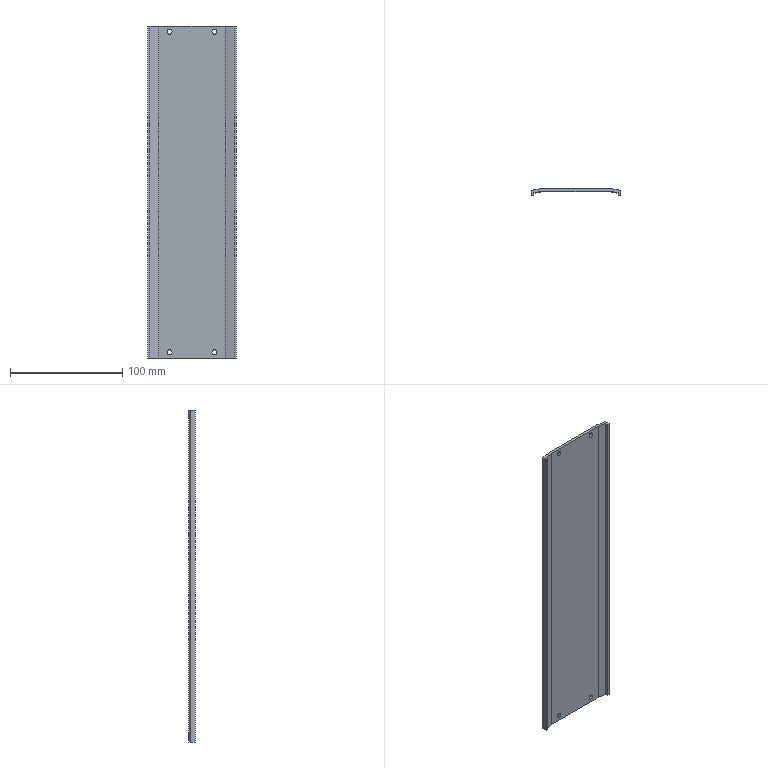Part | SolidWorks | features Cut 1, Extrusion 1, MirrorPattern 1 | 1 solid | 22 faces | box 79 x 6 x 296 mm | volume 60805 mm3 | plane 14 | cylinder 8 | commonest cylinder face diameters 4.5 x8
STEP:
#1=CARTESIAN_POINT('',(20.,3.5,-140.75));
#2=VERTEX_POINT('',#1);
#3=CARTESIAN_POINT('',(20.,3.5,-145.25));
#4=VERTEX_POINT('',#3);
#5=CARTESIAN_POINT('',(20.,3.5,-143.));
#6=DIRECTION('',(0.,-1.,0.));
#7=DIRECTION('',(0.,0.,1.));
#8=AXIS2_PLACEMENT_3D('',#5,#6,#7);
#9=CIRCLE('',#8,2.25);
#10=EDGE_CURVE('',#2,#4,#9,.T.);
#11=ORIENTED_EDGE('',*,*,#10,.T.);
#12=CARTESIAN_POINT('',(20.,6.,-145.25));
#13=VERTEX_POINT('',#12);
#14=CARTESIAN_POINT('',(20.,-4.,-145.25));
#15=DIRECTION('',(0.,1.,0.));
#16=VECTOR('',#15,1000.);
#17=LINE('',#14,#16);
#18=EDGE_CURVE('',#4,#13,#17,.T.);
#19=ORIENTED_EDGE('',*,*,#18,.T.);
#20=CARTESIAN_POINT('',(20.,6.,-140.75));
#21=VERTEX_POINT('',#20);
#22=CARTESIAN_POINT('',(20.,6.,-143.));
#23=DIRECTION('',(0.,-1.,0.));
#24=DIRECTION('',(0.,0.,-1.));
#25=AXIS2_PLACEMENT_3D('',#22,#23,#24);
#26=CIRCLE('',#25,2.25);
#27=EDGE_CURVE('',#21,#13,#26,.T.);
#28=ORIENTED_EDGE('',*,*,#27,.F.);
#29=CARTESIAN_POINT('',(20.,-4.,-140.75));
#30=DIRECTION('',(0.,1.,0.));
#31=VECTOR('',#30,1000.);
#32=LINE('',#29,#31);
#33=EDGE_CURVE('',#2,#21,#32,.T.);
#34=ORIENTED_EDGE('',*,*,#33,.F.);
#35=EDGE_LOOP('',(#11,#19,#28,#34));
#36=FACE_OUTER_BOUND('',#35,.T.);
#37=CARTESIAN_POINT('',(20.,-4.,-143.));
#38=DIRECTION('',(0.,1.,0.));
#39=DIRECTION('',(0.,0.,1.));
#40=AXIS2_PLACEMENT_3D('',#37,#38,#39);
#41=CYLINDRICAL_SURFACE('',#40,2.25);
#42=ADVANCED_FACE('',(#36),#41,.F.);
#43=CARTESIAN_POINT('',(-20.,3.5,-140.75));
#44=VERTEX_POINT('',#43);
#45=CARTESIAN_POINT('',(-20.,3.5,-145.25));
#46=VERTEX_POINT('',#45);
#47=CARTESIAN_POINT('',(-20.,3.5,-143.));
#48=DIRECTION('',(0.,-1.,0.));
#49=DIRECTION('',(0.,0.,1.));
#50=AXIS2_PLACEMENT_3D('',#47,#48,#49);
#51=CIRCLE('',#50,2.25);
#52=EDGE_CURVE('',#44,#46,#51,.T.);
#53=ORIENTED_EDGE('',*,*,#52,.T.);
#54=CARTESIAN_POINT('',(-20.,6.,-145.25));
#55=VERTEX_POINT('',#54);
#56=CARTESIAN_POINT('',(-20.,-4.,-145.25));
#57=DIRECTION('',(0.,1.,0.));
#58=VECTOR('',#57,1000.);
#59=LINE('',#56,#58);
#60=EDGE_CURVE('',#46,#55,#59,.T.);
#61=ORIENTED_EDGE('',*,*,#60,.T.);
#62=CARTESIAN_POINT('',(-20.,6.,-140.75));
#63=VERTEX_POINT('',#62);
#64=CARTESIAN_POINT('',(-20.,6.,-143.));
#65=DIRECTION('',(0.,-1.,0.));
#66=DIRECTION('',(0.,0.,-1.));
#67=AXIS2_PLACEMENT_3D('',#64,#65,#66);
#68=CIRCLE('',#67,2.25);
#69=EDGE_CURVE('',#63,#55,#68,.T.);
#70=ORIENTED_EDGE('',*,*,#69,.F.);
#71=CARTESIAN_POINT('',(-20.,-4.,-140.75));
#72=DIRECTION('',(0.,1.,0.));
#73=VECTOR('',#72,1000.);
#74=LINE('',#71,#73);
#75=EDGE_CURVE('',#44,#63,#74,.T.);
#76=ORIENTED_EDGE('',*,*,#75,.F.);
#77=EDGE_LOOP('',(#53,#61,#70,#76));
#78=FACE_OUTER_BOUND('',#77,.T.);
#79=CARTESIAN_POINT('',(-20.,-4.,-143.));
#80=DIRECTION('',(0.,1.,0.));
#81=DIRECTION('',(0.,0.,1.));
#82=AXIS2_PLACEMENT_3D('',#79,#80,#81);
#83=CYLINDRICAL_SURFACE('',#82,2.25);
#84=ADVANCED_FACE('',(#78),#83,.F.);
#85=CARTESIAN_POINT('',(20.,3.5,140.75));
#86=VERTEX_POINT('',#85);
#87=CARTESIAN_POINT('',(20.,3.5,145.25));
#88=VERTEX_POINT('',#87);
#89=CARTESIAN_POINT('',(20.,3.5,143.));
#90=DIRECTION('',(0.,1.,0.));
#91=DIRECTION('',(0.,0.,1.));
#92=AXIS2_PLACEMENT_3D('',#89,#90,#91);
#93=CIRCLE('',#92,2.25);
#94=EDGE_CURVE('',#86,#88,#93,.T.);
#95=ORIENTED_EDGE('',*,*,#94,.F.);
#96=CARTESIAN_POINT('',(20.,6.,140.75));
#97=VERTEX_POINT('',#96);
#98=CARTESIAN_POINT('',(20.,-4.,140.75));
#99=DIRECTION('',(0.,1.,0.));
#100=VECTOR('',#99,1000.);
#101=LINE('',#98,#100);
#102=EDGE_CURVE('',#86,#97,#101,.T.);
#103=ORIENTED_EDGE('',*,*,#102,.T.);
#104=CARTESIAN_POINT('',(20.,6.,145.25));
#105=VERTEX_POINT('',#104);
#106=CARTESIAN_POINT('',(20.,6.,143.));
#107=DIRECTION('',(0.,1.,0.));
#108=DIRECTION('',(0.,0.,1.));
#109=AXIS2_PLACEMENT_3D('',#106,#107,#108);
#110=CIRCLE('',#109,2.25);
#111=EDGE_CURVE('',#97,#105,#110,.T.);
#112=ORIENTED_EDGE('',*,*,#111,.T.);
#113=CARTESIAN_POINT('',(20.,-4.,145.25));
#114=DIRECTION('',(0.,1.,0.));
#115=VECTOR('',#114,1000.);
#116=LINE('',#113,#115);
#117=EDGE_CURVE('',#88,#105,#116,.T.);
#118=ORIENTED_EDGE('',*,*,#117,.F.);
#119=EDGE_LOOP('',(#95,#103,#112,#118));
#120=FACE_OUTER_BOUND('',#119,.T.);
#121=CARTESIAN_POINT('',(20.,-4.,143.));
#122=DIRECTION('',(0.,1.,0.));
#123=DIRECTION('',(0.,0.,1.));
#124=AXIS2_PLACEMENT_3D('',#121,#122,#123);
#125=CYLINDRICAL_SURFACE('',#124,2.25);
#126=ADVANCED_FACE('',(#120),#125,.F.);
#127=CARTESIAN_POINT('',(-20.,3.5,140.75));
#128=VERTEX_POINT('',#127);
#129=CARTESIAN_POINT('',(-20.,3.5,145.25));
#130=VERTEX_POINT('',#129);
#131=CARTESIAN_POINT('',(-20.,3.5,143.));
#132=DIRECTION('',(0.,1.,0.));
#133=DIRECTION('',(0.,0.,1.));
#134=AXIS2_PLACEMENT_3D('',#131,#132,#133);
#135=CIRCLE('',#134,2.25);
#136=EDGE_CURVE('',#128,#130,#135,.T.);
#137=ORIENTED_EDGE('',*,*,#136,.F.);
#138=CARTESIAN_POINT('',(-20.,6.,140.75));
#139=VERTEX_POINT('',#138);
#140=CARTESIAN_POINT('',(-20.,-4.,140.75));
#141=DIRECTION('',(0.,1.,0.));
#142=VECTOR('',#141,1000.);
#143=LINE('',#140,#142);
#144=EDGE_CURVE('',#128,#139,#143,.T.);
#145=ORIENTED_EDGE('',*,*,#144,.T.);
#146=CARTESIAN_POINT('',(-20.,6.,145.25));
#147=VERTEX_POINT('',#146);
#148=CARTESIAN_POINT('',(-20.,6.,143.));
#149=DIRECTION('',(0.,1.,0.));
#150=DIRECTION('',(0.,0.,1.));
#151=AXIS2_PLACEMENT_3D('',#148,#149,#150);
#152=CIRCLE('',#151,2.25);
#153=EDGE_CURVE('',#139,#147,#152,.T.);
#154=ORIENTED_EDGE('',*,*,#153,.T.);
#155=CARTESIAN_POINT('',(-20.,-4.,145.25));
#156=DIRECTION('',(0.,1.,0.));
#157=VECTOR('',#156,1000.);
#158=LINE('',#155,#157);
#159=EDGE_CURVE('',#130,#147,#158,.T.);
#160=ORIENTED_EDGE('',*,*,#159,.F.);
#161=EDGE_LOOP('',(#137,#145,#154,#160));
#162=FACE_OUTER_BOUND('',#161,.T.);
#163=CARTESIAN_POINT('',(-20.,-4.,143.));
#164=DIRECTION('',(0.,1.,0.));
#165=DIRECTION('',(0.,0.,1.));
#166=AXIS2_PLACEMENT_3D('',#163,#164,#165);
#167=CYLINDRICAL_SURFACE('',#166,2.25);
#168=ADVANCED_FACE('',(#162),#167,.F.);
#169=CARTESIAN_POINT('',(-37.5,0.,-148.));
#170=VERTEX_POINT('',#169);
#171=CARTESIAN_POINT('',(-37.5,2.122,-148.));
#172=VERTEX_POINT('',#171);
#173=CARTESIAN_POINT('',(-37.5,0.,-148.));
#174=DIRECTION('',(0.,1.,0.));
#175=VECTOR('',#174,1000.);
#176=LINE('',#173,#175);
#177=EDGE_CURVE('',#170,#172,#176,.T.);
#178=ORIENTED_EDGE('',*,*,#177,.T.);
#179=CARTESIAN_POINT('',(-37.5,2.122,148.));
#180=VERTEX_POINT('',#179);
#181=CARTESIAN_POINT('',(-37.5,2.122,148.));
#182=DIRECTION('',(0.,0.,-1.));
#183=VECTOR('',#182,1000.);
#184=LINE('',#181,#183);
#185=EDGE_CURVE('',#180,#172,#184,.T.);
#186=ORIENTED_EDGE('',*,*,#185,.F.);
#187=CARTESIAN_POINT('',(-37.5,0.,148.));
#188=VERTEX_POINT('',#187);
#189=CARTESIAN_POINT('',(-37.5,0.,148.));
#190=DIRECTION('',(0.,1.,0.));
#191=VECTOR('',#190,1000.);
#192=LINE('',#189,#191);
#193=EDGE_CURVE('',#188,#180,#192,.T.);
#194=ORIENTED_EDGE('',*,*,#193,.F.);
#195=CARTESIAN_POINT('',(-37.5,0.,148.));
#196=DIRECTION('',(0.,0.,-1.));
#197=VECTOR('',#196,1000.);
#198=LINE('',#195,#197);
#199=EDGE_CURVE('',#188,#170,#198,.T.);
#200=ORIENTED_EDGE('',*,*,#199,.T.);
#201=EDGE_LOOP('',(#178,#186,#194,#200));
#202=FACE_OUTER_BOUND('',#201,.T.);
#203=CARTESIAN_POINT('',(-37.5,0.,148.));
#204=DIRECTION('',(-1.,0.,0.));
#205=DIRECTION('',(0.,0.,1.));
#206=AXIS2_PLACEMENT_3D('',#203,#204,#205);
#207=PLANE('',#206);
#208=ADVANCED_FACE('',(#202),#207,.F.);
#209=CARTESIAN_POINT('',(-29.8,3.5,-148.));
#210=VERTEX_POINT('',#209);
#211=CARTESIAN_POINT('',(-37.5,2.122,-148.));
#212=DIRECTION('',(0.9844,0.1761,0.));
#213=VECTOR('',#212,1000.);
#214=LINE('',#211,#213);
#215=EDGE_CURVE('',#172,#210,#214,.T.);
#216=ORIENTED_EDGE('',*,*,#215,.T.);
#217=CARTESIAN_POINT('',(-29.8,3.5,148.));
#218=VERTEX_POINT('',#217);
#219=CARTESIAN_POINT('',(-29.8,3.5,148.));
#220=DIRECTION('',(0.,0.,-1.));
#221=VECTOR('',#220,1000.);
#222=LINE('',#219,#221);
#223=EDGE_CURVE('',#218,#210,#222,.T.);
#224=ORIENTED_EDGE('',*,*,#223,.F.);
#225=CARTESIAN_POINT('',(-37.5,2.122,148.));
#226=DIRECTION('',(0.9844,0.1761,0.));
#227=VECTOR('',#226,1000.);
#228=LINE('',#225,#227);
#229=EDGE_CURVE('',#180,#218,#228,.T.);
#230=ORIENTED_EDGE('',*,*,#229,.F.);
#231=ORIENTED_EDGE('',*,*,#185,.T.);
#232=EDGE_LOOP('',(#216,#224,#230,#231));
#233=FACE_OUTER_BOUND('',#232,.T.);
#234=CARTESIAN_POINT('',(-37.5,2.122,148.));
#235=DIRECTION('',(-0.1761,0.9844,0.));
#236=DIRECTION('',(-0.9844,-0.1761,0.));
#237=AXIS2_PLACEMENT_3D('',#234,#235,#236);
#238=PLANE('',#237);
#239=ADVANCED_FACE('',(#233),#238,.F.);
#240=ORIENTED_EDGE('',*,*,#10,.F.);
#241=CARTESIAN_POINT('',(20.,3.5,-143.));
#242=DIRECTION('',(0.,-1.,0.));
#243=DIRECTION('',(0.,0.,1.));
#244=AXIS2_PLACEMENT_3D('',#241,#242,#243);
#245=CIRCLE('',#244,2.25);
#246=EDGE_CURVE('',#4,#2,#245,.T.);
#247=ORIENTED_EDGE('',*,*,#246,.F.);
#248=EDGE_LOOP('',(#240,#247));
#249=FACE_BOUND('',#248,.T.);
#250=ORIENTED_EDGE('',*,*,#52,.F.);
#251=CARTESIAN_POINT('',(-20.,3.5,-143.));
#252=DIRECTION('',(0.,-1.,0.));
#253=DIRECTION('',(0.,0.,1.));
#254=AXIS2_PLACEMENT_3D('',#251,#252,#253);
#255=CIRCLE('',#254,2.25);
#256=EDGE_CURVE('',#46,#44,#255,.T.);
#257=ORIENTED_EDGE('',*,*,#256,.F.);
#258=EDGE_LOOP('',(#250,#257));
#259=FACE_BOUND('',#258,.T.);
#260=CARTESIAN_POINT('',(20.,3.5,143.));
#261=DIRECTION('',(0.,1.,0.));
#262=DIRECTION('',(0.,0.,1.));
#263=AXIS2_PLACEMENT_3D('',#260,#261,#262);
#264=CIRCLE('',#263,2.25);
#265=EDGE_CURVE('',#88,#86,#264,.T.);
#266=ORIENTED_EDGE('',*,*,#265,.T.);
#267=ORIENTED_EDGE('',*,*,#94,.T.);
#268=EDGE_LOOP('',(#266,#267));
#269=FACE_BOUND('',#268,.T.);
#270=CARTESIAN_POINT('',(-20.,3.5,143.));
#271=DIRECTION('',(0.,1.,0.));
#272=DIRECTION('',(0.,0.,1.));
#273=AXIS2_PLACEMENT_3D('',#270,#271,#272);
#274=CIRCLE('',#273,2.25);
#275=EDGE_CURVE('',#130,#128,#274,.T.);
#276=ORIENTED_EDGE('',*,*,#275,.T.);
#277=ORIENTED_EDGE('',*,*,#136,.T.);
#278=EDGE_LOOP('',(#276,#277));
#279=FACE_BOUND('',#278,.T.);
#280=CARTESIAN_POINT('',(29.8,3.5,-148.));
#281=VERTEX_POINT('',#280);
#282=CARTESIAN_POINT('',(-29.8,3.5,-148.));
#283=DIRECTION('',(1.,0.,0.));
#284=VECTOR('',#283,1000.);
#285=LINE('',#282,#284);
#286=EDGE_CURVE('',#210,#281,#285,.T.);
#287=ORIENTED_EDGE('',*,*,#286,.T.);
#288=CARTESIAN_POINT('',(29.8,3.5,148.));
#289=VERTEX_POINT('',#288);
#290=CARTESIAN_POINT('',(29.8,3.5,148.));
#291=DIRECTION('',(0.,0.,-1.));
#292=VECTOR('',#291,1000.);
#293=LINE('',#290,#292);
#294=EDGE_CURVE('',#289,#281,#293,.T.);
#295=ORIENTED_EDGE('',*,*,#294,.F.);
#296=CARTESIAN_POINT('',(-29.8,3.5,148.));
#297=DIRECTION('',(1.,0.,0.));
#298=VECTOR('',#297,1000.);
#299=LINE('',#296,#298);
#300=EDGE_CURVE('',#218,#289,#299,.T.);
#301=ORIENTED_EDGE('',*,*,#300,.F.);
#302=ORIENTED_EDGE('',*,*,#223,.T.);
#303=EDGE_LOOP('',(#287,#295,#301,#302));
#304=FACE_OUTER_BOUND('',#303,.T.);
#305=CARTESIAN_POINT('',(-29.8,3.5,148.));
#306=DIRECTION('',(0.,1.,0.));
#307=DIRECTION('',(0.,0.,1.));
#308=AXIS2_PLACEMENT_3D('',#305,#306,#307);
#309=PLANE('',#308);
#310=ADVANCED_FACE('',(#249,#259,#269,#279,#304),#309,.F.);
#311=CARTESIAN_POINT('',(37.5,2.122,-148.));
#312=VERTEX_POINT('',#311);
#313=CARTESIAN_POINT('',(37.5,2.122,-148.));
#314=DIRECTION('',(0.9844,-0.1761,0.));
#315=VECTOR('',#314,1000.);
#316=LINE('',#313,#315);
#317=EDGE_CURVE('',#281,#312,#316,.T.);
#318=ORIENTED_EDGE('',*,*,#317,.T.);
#319=CARTESIAN_POINT('',(37.5,2.122,148.));
#320=VERTEX_POINT('',#319);
#321=CARTESIAN_POINT('',(37.5,2.122,148.));
#322=DIRECTION('',(0.,0.,-1.));
#323=VECTOR('',#322,1000.);
#324=LINE('',#321,#323);
#325=EDGE_CURVE('',#320,#312,#324,.T.);
#326=ORIENTED_EDGE('',*,*,#325,.F.);
#327=CARTESIAN_POINT('',(37.5,2.122,148.));
#328=DIRECTION('',(0.9844,-0.1761,0.));
#329=VECTOR('',#328,1000.);
#330=LINE('',#327,#329);
#331=EDGE_CURVE('',#289,#320,#330,.T.);
#332=ORIENTED_EDGE('',*,*,#331,.F.);
#333=ORIENTED_EDGE('',*,*,#294,.T.);
#334=EDGE_LOOP('',(#318,#326,#332,#333));
#335=FACE_OUTER_BOUND('',#334,.T.);
#336=CARTESIAN_POINT('',(37.5,2.122,148.));
#337=DIRECTION('',(0.1761,0.9844,0.));
#338=DIRECTION('',(-0.9844,0.1761,0.));
#339=AXIS2_PLACEMENT_3D('',#336,#337,#338);
#340=PLANE('',#339);
#341=ADVANCED_FACE('',(#335),#340,.F.);
#342=CARTESIAN_POINT('',(37.5,0.,-148.));
#343=VERTEX_POINT('',#342);
#344=CARTESIAN_POINT('',(37.5,0.,-148.));
#345=DIRECTION('',(0.,-1.,0.));
#346=VECTOR('',#345,1000.);
#347=LINE('',#344,#346);
#348=EDGE_CURVE('',#312,#343,#347,.T.);
#349=ORIENTED_EDGE('',*,*,#348,.T.);
#350=CARTESIAN_POINT('',(37.5,0.,148.));
#351=VERTEX_POINT('',#350);
#352=CARTESIAN_POINT('',(37.5,0.,148.));
#353=DIRECTION('',(0.,0.,-1.));
#354=VECTOR('',#353,1000.);
#355=LINE('',#352,#354);
#356=EDGE_CURVE('',#351,#343,#355,.T.);
#357=ORIENTED_EDGE('',*,*,#356,.F.);
#358=CARTESIAN_POINT('',(37.5,0.,148.));
#359=DIRECTION('',(0.,-1.,0.));
#360=VECTOR('',#359,1000.);
#361=LINE('',#358,#360);
#362=EDGE_CURVE('',#320,#351,#361,.T.);
#363=ORIENTED_EDGE('',*,*,#362,.F.);
#364=ORIENTED_EDGE('',*,*,#325,.T.);
#365=EDGE_LOOP('',(#349,#357,#363,#364));
#366=FACE_OUTER_BOUND('',#365,.T.);
#367=CARTESIAN_POINT('',(37.5,0.,148.));
#368=DIRECTION('',(1.,0.,0.));
#369=DIRECTION('',(0.,0.,-1.));
#370=AXIS2_PLACEMENT_3D('',#367,#368,#369);
#371=PLANE('',#370);
#372=ADVANCED_FACE('',(#366),#371,.F.);
#373=CARTESIAN_POINT('',(39.5,0.,-148.));
#374=VERTEX_POINT('',#373);
#375=CARTESIAN_POINT('',(37.5,0.,-148.));
#376=DIRECTION('',(1.,0.,0.));
#377=VECTOR('',#376,1000.);
#378=LINE('',#375,#377);
#379=EDGE_CURVE('',#343,#374,#378,.T.);
#380=ORIENTED_EDGE('',*,*,#379,.T.);
#381=CARTESIAN_POINT('',(39.5,0.,148.));
#382=VERTEX_POINT('',#381);
#383=CARTESIAN_POINT('',(39.5,0.,148.));
#384=DIRECTION('',(0.,0.,-1.));
#385=VECTOR('',#384,1000.);
#386=LINE('',#383,#385);
#387=EDGE_CURVE('',#382,#374,#386,.T.);
#388=ORIENTED_EDGE('',*,*,#387,.F.);
#389=CARTESIAN_POINT('',(37.5,0.,148.));
#390=DIRECTION('',(1.,0.,0.));
#391=VECTOR('',#390,1000.);
#392=LINE('',#389,#391);
#393=EDGE_CURVE('',#351,#382,#392,.T.);
#394=ORIENTED_EDGE('',*,*,#393,.F.);
#395=ORIENTED_EDGE('',*,*,#356,.T.);
#396=EDGE_LOOP('',(#380,#388,#394,#395));
#397=FACE_OUTER_BOUND('',#396,.T.);
#398=CARTESIAN_POINT('',(37.5,0.,148.));
#399=DIRECTION('',(0.,1.,0.));
#400=DIRECTION('',(-1.,0.,0.));
#401=AXIS2_PLACEMENT_3D('',#398,#399,#400);
#402=PLANE('',#401);
#403=ADVANCED_FACE('',(#397),#402,.F.);
#404=CARTESIAN_POINT('',(39.5,4.3,-148.));
#405=VERTEX_POINT('',#404);
#406=CARTESIAN_POINT('',(39.5,0.,-148.));
#407=DIRECTION('',(0.,1.,0.));
#408=VECTOR('',#407,1000.);
#409=LINE('',#406,#408);
#410=EDGE_CURVE('',#374,#405,#409,.T.);
#411=ORIENTED_EDGE('',*,*,#410,.T.);
#412=CARTESIAN_POINT('',(39.5,4.3,148.));
#413=VERTEX_POINT('',#412);
#414=CARTESIAN_POINT('',(39.5,4.3,148.));
#415=DIRECTION('',(0.,0.,-1.));
#416=VECTOR('',#415,1000.);
#417=LINE('',#414,#416);
#418=EDGE_CURVE('',#413,#405,#417,.T.);
#419=ORIENTED_EDGE('',*,*,#418,.F.);
#420=CARTESIAN_POINT('',(39.5,0.,148.));
#421=DIRECTION('',(0.,1.,0.));
#422=VECTOR('',#421,1000.);
#423=LINE('',#420,#422);
#424=EDGE_CURVE('',#382,#413,#423,.T.);
#425=ORIENTED_EDGE('',*,*,#424,.F.);
#426=ORIENTED_EDGE('',*,*,#387,.T.);
#427=EDGE_LOOP('',(#411,#419,#425,#426));
#428=FACE_OUTER_BOUND('',#427,.T.);
#429=CARTESIAN_POINT('',(39.5,0.,148.));
#430=DIRECTION('',(-1.,0.,0.));
#431=DIRECTION('',(0.,0.,1.));
#432=AXIS2_PLACEMENT_3D('',#429,#430,#431);
#433=PLANE('',#432);
#434=ADVANCED_FACE('',(#428),#433,.F.);
#435=CARTESIAN_POINT('',(30.,6.,-148.));
#436=VERTEX_POINT('',#435);
#437=CARTESIAN_POINT('',(39.5,4.3,-148.));
#438=DIRECTION('',(-0.9844,0.1761,0.));
#439=VECTOR('',#438,1000.);
#440=LINE('',#437,#439);
#441=EDGE_CURVE('',#405,#436,#440,.T.);
#442=ORIENTED_EDGE('',*,*,#441,.T.);
#443=CARTESIAN_POINT('',(30.,6.,148.));
#444=VERTEX_POINT('',#443);
#445=CARTESIAN_POINT('',(30.,6.,148.));
#446=DIRECTION('',(0.,0.,-1.));
#447=VECTOR('',#446,1000.);
#448=LINE('',#445,#447);
#449=EDGE_CURVE('',#444,#436,#448,.T.);
#450=ORIENTED_EDGE('',*,*,#449,.F.);
#451=CARTESIAN_POINT('',(39.5,4.3,148.));
#452=DIRECTION('',(-0.9844,0.1761,0.));
#453=VECTOR('',#452,1000.);
#454=LINE('',#451,#453);
#455=EDGE_CURVE('',#413,#444,#454,.T.);
#456=ORIENTED_EDGE('',*,*,#455,.F.);
#457=ORIENTED_EDGE('',*,*,#418,.T.);
#458=EDGE_LOOP('',(#442,#450,#456,#457));
#459=FACE_OUTER_BOUND('',#458,.T.);
#460=CARTESIAN_POINT('',(39.5,4.3,148.));
#461=DIRECTION('',(-0.1761,-0.9844,0.));
#462=DIRECTION('',(0.9844,-0.1761,0.));
#463=AXIS2_PLACEMENT_3D('',#460,#461,#462);
#464=PLANE('',#463);
#465=ADVANCED_FACE('',(#459),#464,.F.);
#466=ORIENTED_EDGE('',*,*,#27,.T.);
#467=CARTESIAN_POINT('',(20.,6.,-143.));
#468=DIRECTION('',(0.,-1.,0.));
#469=DIRECTION('',(0.,0.,-1.));
#470=AXIS2_PLACEMENT_3D('',#467,#468,#469);
#471=CIRCLE('',#470,2.25);
#472=EDGE_CURVE('',#13,#21,#471,.T.);
#473=ORIENTED_EDGE('',*,*,#472,.T.);
#474=EDGE_LOOP('',(#466,#473));
#475=FACE_BOUND('',#474,.T.);
#476=ORIENTED_EDGE('',*,*,#69,.T.);
#477=CARTESIAN_POINT('',(-20.,6.,-143.));
#478=DIRECTION('',(0.,-1.,0.));
#479=DIRECTION('',(0.,0.,-1.));
#480=AXIS2_PLACEMENT_3D('',#477,#478,#479);
#481=CIRCLE('',#480,2.25);
#482=EDGE_CURVE('',#55,#63,#481,.T.);
#483=ORIENTED_EDGE('',*,*,#482,.T.);
#484=EDGE_LOOP('',(#476,#483));
#485=FACE_BOUND('',#484,.T.);
#486=CARTESIAN_POINT('',(20.,6.,143.));
#487=DIRECTION('',(0.,1.,0.));
#488=DIRECTION('',(0.,0.,1.));
#489=AXIS2_PLACEMENT_3D('',#486,#487,#488);
#490=CIRCLE('',#489,2.25);
#491=EDGE_CURVE('',#105,#97,#490,.T.);
#492=ORIENTED_EDGE('',*,*,#491,.F.);
#493=ORIENTED_EDGE('',*,*,#111,.F.);
#494=EDGE_LOOP('',(#492,#493));
#495=FACE_BOUND('',#494,.T.);
#496=CARTESIAN_POINT('',(-20.,6.,143.));
#497=DIRECTION('',(0.,1.,0.));
#498=DIRECTION('',(0.,0.,1.));
#499=AXIS2_PLACEMENT_3D('',#496,#497,#498);
#500=CIRCLE('',#499,2.25);
#501=EDGE_CURVE('',#147,#139,#500,.T.);
#502=ORIENTED_EDGE('',*,*,#501,.F.);
#503=ORIENTED_EDGE('',*,*,#153,.F.);
#504=EDGE_LOOP('',(#502,#503));
#505=FACE_BOUND('',#504,.T.);
#506=CARTESIAN_POINT('',(-30.,6.,-148.));
#507=VERTEX_POINT('',#506);
#508=CARTESIAN_POINT('',(-30.,6.,-148.));
#509=DIRECTION('',(-1.,0.,0.));
#510=VECTOR('',#509,1000.);
#511=LINE('',#508,#510);
#512=EDGE_CURVE('',#436,#507,#511,.T.);
#513=ORIENTED_EDGE('',*,*,#512,.T.);
#514=CARTESIAN_POINT('',(-30.,6.,148.));
#515=VERTEX_POINT('',#514);
#516=CARTESIAN_POINT('',(-30.,6.,148.));
#517=DIRECTION('',(0.,0.,-1.));
#518=VECTOR('',#517,1000.);
#519=LINE('',#516,#518);
#520=EDGE_CURVE('',#515,#507,#519,.T.);
#521=ORIENTED_EDGE('',*,*,#520,.F.);
#522=CARTESIAN_POINT('',(-30.,6.,148.));
#523=DIRECTION('',(-1.,0.,0.));
#524=VECTOR('',#523,1000.);
#525=LINE('',#522,#524);
#526=EDGE_CURVE('',#444,#515,#525,.T.);
#527=ORIENTED_EDGE('',*,*,#526,.F.);
#528=ORIENTED_EDGE('',*,*,#449,.T.);
#529=EDGE_LOOP('',(#513,#521,#527,#528));
#530=FACE_OUTER_BOUND('',#529,.T.);
#531=CARTESIAN_POINT('',(-30.,6.,148.));
#532=DIRECTION('',(0.,-1.,0.));
#533=DIRECTION('',(0.,0.,-1.));
#534=AXIS2_PLACEMENT_3D('',#531,#532,#533);
#535=PLANE('',#534);
#536=ADVANCED_FACE('',(#475,#485,#495,#505,#530),#535,.F.);
#537=CARTESIAN_POINT('',(-39.5,4.3,-148.));
#538=VERTEX_POINT('',#537);
#539=CARTESIAN_POINT('',(-39.5,4.3,-148.));
#540=DIRECTION('',(-0.9844,-0.1761,0.));
#541=VECTOR('',#540,1000.);
#542=LINE('',#539,#541);
#543=EDGE_CURVE('',#507,#538,#542,.T.);
#544=ORIENTED_EDGE('',*,*,#543,.T.);
#545=CARTESIAN_POINT('',(-39.5,4.3,148.));
#546=VERTEX_POINT('',#545);
#547=CARTESIAN_POINT('',(-39.5,4.3,148.));
#548=DIRECTION('',(0.,0.,-1.));
#549=VECTOR('',#548,1000.);
#550=LINE('',#547,#549);
#551=EDGE_CURVE('',#546,#538,#550,.T.);
#552=ORIENTED_EDGE('',*,*,#551,.F.);
#553=CARTESIAN_POINT('',(-39.5,4.3,148.));
#554=DIRECTION('',(-0.9844,-0.1761,0.));
#555=VECTOR('',#554,1000.);
#556=LINE('',#553,#555);
#557=EDGE_CURVE('',#515,#546,#556,.T.);
#558=ORIENTED_EDGE('',*,*,#557,.F.);
#559=ORIENTED_EDGE('',*,*,#520,.T.);
#560=EDGE_LOOP('',(#544,#552,#558,#559));
#561=FACE_OUTER_BOUND('',#560,.T.);
#562=CARTESIAN_POINT('',(-39.5,4.3,148.));
#563=DIRECTION('',(0.1761,-0.9844,0.));
#564=DIRECTION('',(0.9844,0.1761,0.));
#565=AXIS2_PLACEMENT_3D('',#562,#563,#564);
#566=PLANE('',#565);
#567=ADVANCED_FACE('',(#561),#566,.F.);
#568=CARTESIAN_POINT('',(-39.5,0.,-148.));
#569=VERTEX_POINT('',#568);
#570=CARTESIAN_POINT('',(-39.5,0.,-148.));
#571=DIRECTION('',(0.,-1.,0.));
#572=VECTOR('',#571,1000.);
#573=LINE('',#570,#572);
#574=EDGE_CURVE('',#538,#569,#573,.T.);
#575=ORIENTED_EDGE('',*,*,#574,.T.);
#576=CARTESIAN_POINT('',(-39.5,0.,148.));
#577=VERTEX_POINT('',#576);
#578=CARTESIAN_POINT('',(-39.5,0.,148.));
#579=DIRECTION('',(0.,0.,-1.));
#580=VECTOR('',#579,1000.);
#581=LINE('',#578,#580);
#582=EDGE_CURVE('',#577,#569,#581,.T.);
#583=ORIENTED_EDGE('',*,*,#582,.F.);
#584=CARTESIAN_POINT('',(-39.5,0.,148.));
#585=DIRECTION('',(0.,-1.,0.));
#586=VECTOR('',#585,1000.);
#587=LINE('',#584,#586);
#588=EDGE_CURVE('',#546,#577,#587,.T.);
#589=ORIENTED_EDGE('',*,*,#588,.F.);
#590=ORIENTED_EDGE('',*,*,#551,.T.);
#591=EDGE_LOOP('',(#575,#583,#589,#590));
#592=FACE_OUTER_BOUND('',#591,.T.);
#593=CARTESIAN_POINT('',(-39.5,0.,148.));
#594=DIRECTION('',(1.,0.,0.));
#595=DIRECTION('',(0.,0.,-1.));
#596=AXIS2_PLACEMENT_3D('',#593,#594,#595);
#597=PLANE('',#596);
#598=ADVANCED_FACE('',(#592),#597,.F.);
#599=CARTESIAN_POINT('',(-37.5,0.,-148.));
#600=DIRECTION('',(1.,0.,0.));
#601=VECTOR('',#600,1000.);
#602=LINE('',#599,#601);
#603=EDGE_CURVE('',#569,#170,#602,.T.);
#604=ORIENTED_EDGE('',*,*,#603,.T.);
#605=ORIENTED_EDGE('',*,*,#199,.F.);
#606=CARTESIAN_POINT('',(-37.5,0.,148.));
#607=DIRECTION('',(1.,0.,0.));
#608=VECTOR('',#607,1000.);
#609=LINE('',#606,#608);
#610=EDGE_CURVE('',#577,#188,#609,.T.);
#611=ORIENTED_EDGE('',*,*,#610,.F.);
#612=ORIENTED_EDGE('',*,*,#582,.T.);
#613=EDGE_LOOP('',(#604,#605,#611,#612));
#614=FACE_OUTER_BOUND('',#613,.T.);
#615=CARTESIAN_POINT('',(-37.5,0.,148.));
#616=DIRECTION('',(0.,1.,0.));
#617=DIRECTION('',(-1.,0.,0.));
#618=AXIS2_PLACEMENT_3D('',#615,#616,#617);
#619=PLANE('',#618);
#620=ADVANCED_FACE('',(#614),#619,.F.);
#621=ORIENTED_EDGE('',*,*,#193,.T.);
#622=ORIENTED_EDGE('',*,*,#229,.T.);
#623=ORIENTED_EDGE('',*,*,#300,.T.);
#624=ORIENTED_EDGE('',*,*,#331,.T.);
#625=ORIENTED_EDGE('',*,*,#362,.T.);
#626=ORIENTED_EDGE('',*,*,#393,.T.);
#627=ORIENTED_EDGE('',*,*,#424,.T.);
#628=ORIENTED_EDGE('',*,*,#455,.T.);
#629=ORIENTED_EDGE('',*,*,#526,.T.);
#630=ORIENTED_EDGE('',*,*,#557,.T.);
#631=ORIENTED_EDGE('',*,*,#588,.T.);
#632=ORIENTED_EDGE('',*,*,#610,.T.);
#633=EDGE_LOOP('',(#621,#622,#623,#624,#625,#626,#627,#628,#629,#630,#631,#632));
#634=FACE_OUTER_BOUND('',#633,.T.);
#635=CARTESIAN_POINT('',(0.,0.,148.));
#636=DIRECTION('',(0.,0.,-1.));
#637=DIRECTION('',(-1.,0.,0.));
#638=AXIS2_PLACEMENT_3D('',#635,#636,#637);
#639=PLANE('',#638);
#640=ADVANCED_FACE('',(#634),#639,.F.);
#641=ORIENTED_EDGE('',*,*,#177,.F.);
#642=ORIENTED_EDGE('',*,*,#603,.F.);
#643=ORIENTED_EDGE('',*,*,#574,.F.);
#644=ORIENTED_EDGE('',*,*,#543,.F.);
#645=ORIENTED_EDGE('',*,*,#512,.F.);
#646=ORIENTED_EDGE('',*,*,#441,.F.);
#647=ORIENTED_EDGE('',*,*,#410,.F.);
#648=ORIENTED_EDGE('',*,*,#379,.F.);
#649=ORIENTED_EDGE('',*,*,#348,.F.);
#650=ORIENTED_EDGE('',*,*,#317,.F.);
#651=ORIENTED_EDGE('',*,*,#286,.F.);
#652=ORIENTED_EDGE('',*,*,#215,.F.);
#653=EDGE_LOOP('',(#641,#642,#643,#644,#645,#646,#647,#648,#649,#650,#651,#652));
#654=FACE_OUTER_BOUND('',#653,.T.);
#655=CARTESIAN_POINT('',(0.,0.,-148.));
#656=DIRECTION('',(0.,0.,-1.));
#657=DIRECTION('',(-1.,0.,0.));
#658=AXIS2_PLACEMENT_3D('',#655,#656,#657);
#659=PLANE('',#658);
#660=ADVANCED_FACE('',(#654),#659,.T.);
#661=ORIENTED_EDGE('',*,*,#144,.F.);
#662=ORIENTED_EDGE('',*,*,#275,.F.);
#663=ORIENTED_EDGE('',*,*,#159,.T.);
#664=ORIENTED_EDGE('',*,*,#501,.T.);
#665=EDGE_LOOP('',(#661,#662,#663,#664));
#666=FACE_OUTER_BOUND('',#665,.T.);
#667=CARTESIAN_POINT('',(-20.,-4.,143.));
#668=DIRECTION('',(0.,1.,0.));
#669=DIRECTION('',(0.,0.,1.));
#670=AXIS2_PLACEMENT_3D('',#667,#668,#669);
#671=CYLINDRICAL_SURFACE('',#670,2.25);
#672=ADVANCED_FACE('',(#666),#671,.F.);
#673=ORIENTED_EDGE('',*,*,#102,.F.);
#674=ORIENTED_EDGE('',*,*,#265,.F.);
#675=ORIENTED_EDGE('',*,*,#117,.T.);
#676=ORIENTED_EDGE('',*,*,#491,.T.);
#677=EDGE_LOOP('',(#673,#674,#675,#676));
#678=FACE_OUTER_BOUND('',#677,.T.);
#679=CARTESIAN_POINT('',(20.,-4.,143.));
#680=DIRECTION('',(0.,1.,0.));
#681=DIRECTION('',(0.,0.,1.));
#682=AXIS2_PLACEMENT_3D('',#679,#680,#681);
#683=CYLINDRICAL_SURFACE('',#682,2.25);
#684=ADVANCED_FACE('',(#678),#683,.F.);
#685=ORIENTED_EDGE('',*,*,#60,.F.);
#686=ORIENTED_EDGE('',*,*,#256,.T.);
#687=ORIENTED_EDGE('',*,*,#75,.T.);
#688=ORIENTED_EDGE('',*,*,#482,.F.);
#689=EDGE_LOOP('',(#685,#686,#687,#688));
#690=FACE_OUTER_BOUND('',#689,.T.);
#691=CARTESIAN_POINT('',(-20.,-4.,-143.));
#692=DIRECTION('',(0.,1.,0.));
#693=DIRECTION('',(0.,0.,1.));
#694=AXIS2_PLACEMENT_3D('',#691,#692,#693);
#695=CYLINDRICAL_SURFACE('',#694,2.25);
#696=ADVANCED_FACE('',(#690),#695,.F.);
#697=ORIENTED_EDGE('',*,*,#18,.F.);
#698=ORIENTED_EDGE('',*,*,#246,.T.);
#699=ORIENTED_EDGE('',*,*,#33,.T.);
#700=ORIENTED_EDGE('',*,*,#472,.F.);
#701=EDGE_LOOP('',(#697,#698,#699,#700));
#702=FACE_OUTER_BOUND('',#701,.T.);
#703=CARTESIAN_POINT('',(20.,-4.,-143.));
#704=DIRECTION('',(0.,1.,0.));
#705=DIRECTION('',(0.,0.,1.));
#706=AXIS2_PLACEMENT_3D('',#703,#704,#705);
#707=CYLINDRICAL_SURFACE('',#706,2.25);
#708=ADVANCED_FACE('',(#702),#707,.F.);
#709=CLOSED_SHELL('',(#42,#84,#126,#168,#208,#239,#310,#341,#372,#403,#434,#465,#536,#567,#598,#620,#640,#660,#672,#684,#696,#708));
#710=MANIFOLD_SOLID_BREP('',#709);
#711=CARTESIAN_POINT('',(0.,0.,0.));
#712=DIRECTION('',(0.,0.,1.));
#713=DIRECTION('',(1.,0.,0.));
#714=AXIS2_PLACEMENT_3D('',#711,#712,#713);
#715=(LENGTH_UNIT()NAMED_UNIT(*)SI_UNIT(.MILLI.,.METRE.));
#716=UNCERTAINTY_MEASURE_WITH_UNIT(LENGTH_MEASURE(0.00001),#715,'','');
#717=(NAMED_UNIT(*)PLANE_ANGLE_UNIT()SI_UNIT($,.RADIAN.));
#718=(NAMED_UNIT(*)SI_UNIT($,.STERADIAN.)SOLID_ANGLE_UNIT());
#719=(GEOMETRIC_REPRESENTATION_CONTEXT(3)GLOBAL_UNCERTAINTY_ASSIGNED_CONTEXT((#716))GLOBAL_UNIT_ASSIGNED_CONTEXT((#715,#717,#718))REPRESENTATION_CONTEXT('',''));
#720=ADVANCED_BREP_SHAPE_REPRESENTATION('',(#710,#714),#719);